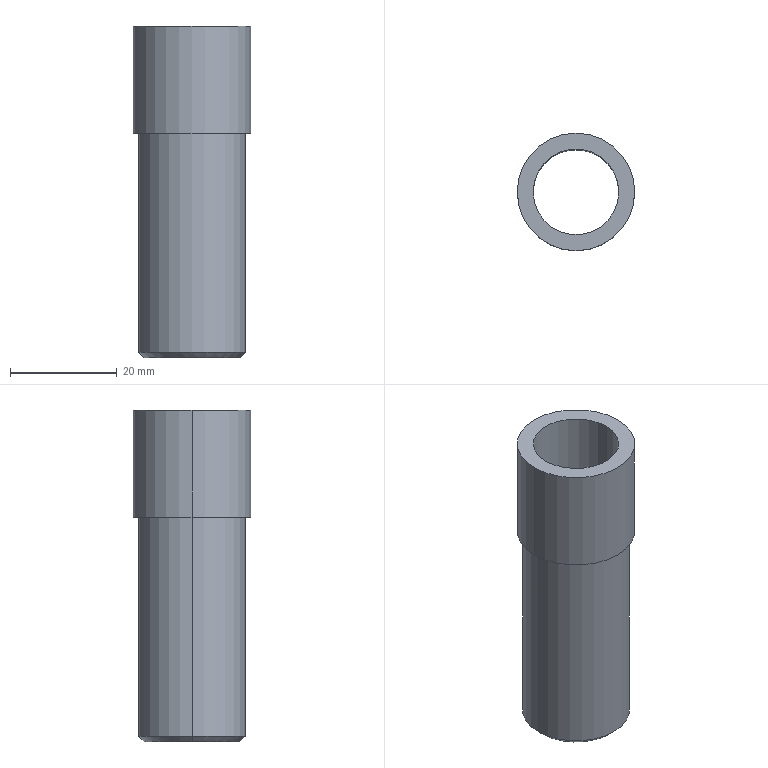Part | SolidWorks | features BaseBody 1 | 1 solid | 11 faces | box 22 x 22 x 62 mm | volume 8301 mm3 | cylinder 6 | plane 3 | cone 2 | commonest cylinder face diameters 16 x2 20 x2 22 x2
STEP:
#1=CARTESIAN_POINT('',(8.,0.,0.));
#2=VERTEX_POINT('',#1);
#3=CARTESIAN_POINT('',(-8.,0.,0.));
#4=VERTEX_POINT('',#3);
#5=CARTESIAN_POINT('',(0.,0.,0.));
#6=DIRECTION('',(0.,0.,-1.));
#7=DIRECTION('',(-1.,0.,0.));
#8=AXIS2_PLACEMENT_3D('',#5,#6,#7);
#9=CIRCLE('',#8,8.);
#10=EDGE_CURVE('',#2,#4,#9,.T.);
#11=ORIENTED_EDGE('',*,*,#10,.F.);
#12=CARTESIAN_POINT('',(8.,0.,-62.));
#13=VERTEX_POINT('',#12);
#14=CARTESIAN_POINT('',(8.,0.,-31.));
#15=DIRECTION('',(0.,0.,-1.));
#16=VECTOR('',#15,1000.);
#17=LINE('',#14,#16);
#18=EDGE_CURVE('',#2,#13,#17,.T.);
#19=ORIENTED_EDGE('',*,*,#18,.T.);
#20=CARTESIAN_POINT('',(-8.,0.,-62.));
#21=VERTEX_POINT('',#20);
#22=CARTESIAN_POINT('',(0.,0.,-62.));
#23=DIRECTION('',(0.,0.,1.));
#24=DIRECTION('',(-1.,0.,0.));
#25=AXIS2_PLACEMENT_3D('',#22,#23,#24);
#26=CIRCLE('',#25,8.);
#27=EDGE_CURVE('',#21,#13,#26,.T.);
#28=ORIENTED_EDGE('',*,*,#27,.F.);
#29=CARTESIAN_POINT('',(-8.,0.,-31.));
#30=DIRECTION('',(0.,0.,-1.));
#31=VECTOR('',#30,1000.);
#32=LINE('',#29,#31);
#33=EDGE_CURVE('',#4,#21,#32,.T.);
#34=ORIENTED_EDGE('',*,*,#33,.F.);
#35=EDGE_LOOP('',(#11,#19,#28,#34));
#36=FACE_OUTER_BOUND('',#35,.T.);
#37=CARTESIAN_POINT('',(0.,0.,-31.));
#38=DIRECTION('',(0.,0.,-1.));
#39=DIRECTION('',(-1.,0.,0.));
#40=AXIS2_PLACEMENT_3D('',#37,#38,#39);
#41=CYLINDRICAL_SURFACE('',#40,8.);
#42=ADVANCED_FACE('',(#36),#41,.F.);
#43=CARTESIAN_POINT('',(11.,0.,0.));
#44=VERTEX_POINT('',#43);
#45=CARTESIAN_POINT('',(-11.,0.,0.));
#46=VERTEX_POINT('',#45);
#47=CARTESIAN_POINT('',(0.,0.,0.));
#48=DIRECTION('',(0.,0.,1.));
#49=DIRECTION('',(-1.,0.,0.));
#50=AXIS2_PLACEMENT_3D('',#47,#48,#49);
#51=CIRCLE('',#50,11.);
#52=EDGE_CURVE('',#44,#46,#51,.T.);
#53=ORIENTED_EDGE('',*,*,#52,.F.);
#54=CARTESIAN_POINT('',(11.,0.,-20.));
#55=VERTEX_POINT('',#54);
#56=CARTESIAN_POINT('',(11.,0.,-10.));
#57=DIRECTION('',(0.,0.,-1.));
#58=VECTOR('',#57,1000.);
#59=LINE('',#56,#58);
#60=EDGE_CURVE('',#44,#55,#59,.T.);
#61=ORIENTED_EDGE('',*,*,#60,.T.);
#62=CARTESIAN_POINT('',(-11.,0.,-20.));
#63=VERTEX_POINT('',#62);
#64=CARTESIAN_POINT('',(0.,0.,-20.));
#65=DIRECTION('',(0.,0.,1.));
#66=DIRECTION('',(-1.,0.,0.));
#67=AXIS2_PLACEMENT_3D('',#64,#65,#66);
#68=CIRCLE('',#67,11.);
#69=EDGE_CURVE('',#55,#63,#68,.T.);
#70=ORIENTED_EDGE('',*,*,#69,.T.);
#71=CARTESIAN_POINT('',(-11.,0.,-10.));
#72=DIRECTION('',(0.,0.,-1.));
#73=VECTOR('',#72,1000.);
#74=LINE('',#71,#73);
#75=EDGE_CURVE('',#46,#63,#74,.T.);
#76=ORIENTED_EDGE('',*,*,#75,.F.);
#77=EDGE_LOOP('',(#53,#61,#70,#76));
#78=FACE_OUTER_BOUND('',#77,.T.);
#79=CARTESIAN_POINT('',(0.,0.,-10.));
#80=DIRECTION('',(0.,0.,-1.));
#81=DIRECTION('',(-1.,0.,0.));
#82=AXIS2_PLACEMENT_3D('',#79,#80,#81);
#83=CYLINDRICAL_SURFACE('',#82,11.);
#84=ADVANCED_FACE('',(#78),#83,.T.);
#85=CARTESIAN_POINT('',(-9.,0.,-62.));
#86=VERTEX_POINT('',#85);
#87=CARTESIAN_POINT('',(9.,0.,-62.));
#88=VERTEX_POINT('',#87);
#89=CARTESIAN_POINT('',(0.,0.,-62.));
#90=DIRECTION('',(0.,0.,-1.));
#91=DIRECTION('',(1.,0.,0.));
#92=AXIS2_PLACEMENT_3D('',#89,#90,#91);
#93=CIRCLE('',#92,9.);
#94=EDGE_CURVE('',#86,#88,#93,.T.);
#95=ORIENTED_EDGE('',*,*,#94,.F.);
#96=CARTESIAN_POINT('',(-10.,0.,-61.));
#97=VERTEX_POINT('',#96);
#98=CARTESIAN_POINT('',(-10.,0.,-61.));
#99=DIRECTION('',(-0.7071,0.,0.7071));
#100=VECTOR('',#99,1000.);
#101=LINE('',#98,#100);
#102=EDGE_CURVE('',#86,#97,#101,.T.);
#103=ORIENTED_EDGE('',*,*,#102,.T.);
#104=CARTESIAN_POINT('',(10.,0.,-61.));
#105=VERTEX_POINT('',#104);
#106=CARTESIAN_POINT('',(0.,0.,-61.));
#107=DIRECTION('',(0.,0.,-1.));
#108=DIRECTION('',(1.,0.,0.));
#109=AXIS2_PLACEMENT_3D('',#106,#107,#108);
#110=CIRCLE('',#109,10.);
#111=EDGE_CURVE('',#97,#105,#110,.T.);
#112=ORIENTED_EDGE('',*,*,#111,.T.);
#113=CARTESIAN_POINT('',(10.,0.,-61.));
#114=DIRECTION('',(0.7071,0.,0.7071));
#115=VECTOR('',#114,1000.);
#116=LINE('',#113,#115);
#117=EDGE_CURVE('',#88,#105,#116,.T.);
#118=ORIENTED_EDGE('',*,*,#117,.F.);
#119=EDGE_LOOP('',(#95,#103,#112,#118));
#120=FACE_OUTER_BOUND('',#119,.T.);
#121=CARTESIAN_POINT('',(0.,0.,-61.));
#122=DIRECTION('',(0.,0.,1.));
#123=DIRECTION('',(1.,0.,0.));
#124=AXIS2_PLACEMENT_3D('',#121,#122,#123);
#125=CONICAL_SURFACE('',#124,10.,0.7854);
#126=ADVANCED_FACE('',(#120),#125,.T.);
#127=CARTESIAN_POINT('',(10.,0.,-20.));
#128=VERTEX_POINT('',#127);
#129=CARTESIAN_POINT('',(-10.,0.,-20.));
#130=VERTEX_POINT('',#129);
#131=CARTESIAN_POINT('',(0.,0.,-20.));
#132=DIRECTION('',(0.,0.,1.));
#133=DIRECTION('',(-1.,0.,0.));
#134=AXIS2_PLACEMENT_3D('',#131,#132,#133);
#135=CIRCLE('',#134,10.);
#136=EDGE_CURVE('',#128,#130,#135,.T.);
#137=ORIENTED_EDGE('',*,*,#136,.F.);
#138=CARTESIAN_POINT('',(10.,0.,-41.));
#139=DIRECTION('',(0.,0.,-1.));
#140=VECTOR('',#139,1000.);
#141=LINE('',#138,#140);
#142=EDGE_CURVE('',#128,#105,#141,.T.);
#143=ORIENTED_EDGE('',*,*,#142,.T.);
#144=ORIENTED_EDGE('',*,*,#111,.F.);
#145=CARTESIAN_POINT('',(-10.,0.,-41.));
#146=DIRECTION('',(0.,0.,-1.));
#147=VECTOR('',#146,1000.);
#148=LINE('',#145,#147);
#149=EDGE_CURVE('',#130,#97,#148,.T.);
#150=ORIENTED_EDGE('',*,*,#149,.F.);
#151=EDGE_LOOP('',(#137,#143,#144,#150));
#152=FACE_OUTER_BOUND('',#151,.T.);
#153=CARTESIAN_POINT('',(0.,0.,-41.));
#154=DIRECTION('',(0.,0.,-1.));
#155=DIRECTION('',(-1.,0.,0.));
#156=AXIS2_PLACEMENT_3D('',#153,#154,#155);
#157=CYLINDRICAL_SURFACE('',#156,10.);
#158=ADVANCED_FACE('',(#152),#157,.T.);
#159=ORIENTED_EDGE('',*,*,#18,.F.);
#160=CARTESIAN_POINT('',(0.,0.,0.));
#161=DIRECTION('',(0.,0.,-1.));
#162=DIRECTION('',(-1.,0.,0.));
#163=AXIS2_PLACEMENT_3D('',#160,#161,#162);
#164=CIRCLE('',#163,8.);
#165=EDGE_CURVE('',#4,#2,#164,.T.);
#166=ORIENTED_EDGE('',*,*,#165,.F.);
#167=ORIENTED_EDGE('',*,*,#33,.T.);
#168=CARTESIAN_POINT('',(0.,0.,-62.));
#169=DIRECTION('',(0.,0.,1.));
#170=DIRECTION('',(-1.,0.,0.));
#171=AXIS2_PLACEMENT_3D('',#168,#169,#170);
#172=CIRCLE('',#171,8.);
#173=EDGE_CURVE('',#13,#21,#172,.T.);
#174=ORIENTED_EDGE('',*,*,#173,.F.);
#175=EDGE_LOOP('',(#159,#166,#167,#174));
#176=FACE_OUTER_BOUND('',#175,.T.);
#177=CARTESIAN_POINT('',(0.,0.,-31.));
#178=DIRECTION('',(0.,0.,-1.));
#179=DIRECTION('',(-1.,0.,0.));
#180=AXIS2_PLACEMENT_3D('',#177,#178,#179);
#181=CYLINDRICAL_SURFACE('',#180,8.);
#182=ADVANCED_FACE('',(#176),#181,.F.);
#183=ORIENTED_EDGE('',*,*,#165,.T.);
#184=ORIENTED_EDGE('',*,*,#10,.T.);
#185=EDGE_LOOP('',(#183,#184));
#186=FACE_BOUND('',#185,.T.);
#187=CARTESIAN_POINT('',(0.,0.,0.));
#188=DIRECTION('',(0.,0.,1.));
#189=DIRECTION('',(-1.,0.,0.));
#190=AXIS2_PLACEMENT_3D('',#187,#188,#189);
#191=CIRCLE('',#190,11.);
#192=EDGE_CURVE('',#46,#44,#191,.T.);
#193=ORIENTED_EDGE('',*,*,#192,.T.);
#194=ORIENTED_EDGE('',*,*,#52,.T.);
#195=EDGE_LOOP('',(#193,#194));
#196=FACE_OUTER_BOUND('',#195,.T.);
#197=CARTESIAN_POINT('',(-11.,0.,0.));
#198=DIRECTION('',(0.,0.,1.));
#199=DIRECTION('',(1.,0.,0.));
#200=AXIS2_PLACEMENT_3D('',#197,#198,#199);
#201=PLANE('',#200);
#202=ADVANCED_FACE('',(#186,#196),#201,.T.);
#203=ORIENTED_EDGE('',*,*,#27,.T.);
#204=ORIENTED_EDGE('',*,*,#173,.T.);
#205=EDGE_LOOP('',(#203,#204));
#206=FACE_BOUND('',#205,.T.);
#207=CARTESIAN_POINT('',(0.,0.,-62.));
#208=DIRECTION('',(0.,0.,-1.));
#209=DIRECTION('',(1.,0.,0.));
#210=AXIS2_PLACEMENT_3D('',#207,#208,#209);
#211=CIRCLE('',#210,9.);
#212=EDGE_CURVE('',#88,#86,#211,.T.);
#213=ORIENTED_EDGE('',*,*,#212,.T.);
#214=ORIENTED_EDGE('',*,*,#94,.T.);
#215=EDGE_LOOP('',(#213,#214));
#216=FACE_OUTER_BOUND('',#215,.T.);
#217=CARTESIAN_POINT('',(-8.,0.,-62.));
#218=DIRECTION('',(0.,0.,-1.));
#219=DIRECTION('',(-1.,0.,0.));
#220=AXIS2_PLACEMENT_3D('',#217,#218,#219);
#221=PLANE('',#220);
#222=ADVANCED_FACE('',(#206,#216),#221,.T.);
#223=ORIENTED_EDGE('',*,*,#60,.F.);
#224=ORIENTED_EDGE('',*,*,#192,.F.);
#225=ORIENTED_EDGE('',*,*,#75,.T.);
#226=CARTESIAN_POINT('',(0.,0.,-20.));
#227=DIRECTION('',(0.,0.,1.));
#228=DIRECTION('',(-1.,0.,0.));
#229=AXIS2_PLACEMENT_3D('',#226,#227,#228);
#230=CIRCLE('',#229,11.);
#231=EDGE_CURVE('',#63,#55,#230,.T.);
#232=ORIENTED_EDGE('',*,*,#231,.T.);
#233=EDGE_LOOP('',(#223,#224,#225,#232));
#234=FACE_OUTER_BOUND('',#233,.T.);
#235=CARTESIAN_POINT('',(0.,0.,-10.));
#236=DIRECTION('',(0.,0.,-1.));
#237=DIRECTION('',(-1.,0.,0.));
#238=AXIS2_PLACEMENT_3D('',#235,#236,#237);
#239=CYLINDRICAL_SURFACE('',#238,11.);
#240=ADVANCED_FACE('',(#234),#239,.T.);
#241=ORIENTED_EDGE('',*,*,#102,.F.);
#242=ORIENTED_EDGE('',*,*,#212,.F.);
#243=ORIENTED_EDGE('',*,*,#117,.T.);
#244=CARTESIAN_POINT('',(0.,0.,-61.));
#245=DIRECTION('',(0.,0.,-1.));
#246=DIRECTION('',(1.,0.,0.));
#247=AXIS2_PLACEMENT_3D('',#244,#245,#246);
#248=CIRCLE('',#247,10.);
#249=EDGE_CURVE('',#105,#97,#248,.T.);
#250=ORIENTED_EDGE('',*,*,#249,.T.);
#251=EDGE_LOOP('',(#241,#242,#243,#250));
#252=FACE_OUTER_BOUND('',#251,.T.);
#253=CARTESIAN_POINT('',(0.,0.,-61.));
#254=DIRECTION('',(0.,0.,1.));
#255=DIRECTION('',(1.,0.,0.));
#256=AXIS2_PLACEMENT_3D('',#253,#254,#255);
#257=CONICAL_SURFACE('',#256,10.,0.7854);
#258=ADVANCED_FACE('',(#252),#257,.T.);
#259=CARTESIAN_POINT('',(0.,0.,-20.));
#260=DIRECTION('',(0.,0.,1.));
#261=DIRECTION('',(-1.,0.,0.));
#262=AXIS2_PLACEMENT_3D('',#259,#260,#261);
#263=CIRCLE('',#262,10.);
#264=EDGE_CURVE('',#130,#128,#263,.T.);
#265=ORIENTED_EDGE('',*,*,#264,.T.);
#266=ORIENTED_EDGE('',*,*,#136,.T.);
#267=EDGE_LOOP('',(#265,#266));
#268=FACE_BOUND('',#267,.T.);
#269=ORIENTED_EDGE('',*,*,#231,.F.);
#270=ORIENTED_EDGE('',*,*,#69,.F.);
#271=EDGE_LOOP('',(#269,#270));
#272=FACE_OUTER_BOUND('',#271,.T.);
#273=CARTESIAN_POINT('',(-10.,0.,-20.));
#274=DIRECTION('',(0.,0.,-1.));
#275=DIRECTION('',(-1.,0.,0.));
#276=AXIS2_PLACEMENT_3D('',#273,#274,#275);
#277=PLANE('',#276);
#278=ADVANCED_FACE('',(#268,#272),#277,.T.);
#279=ORIENTED_EDGE('',*,*,#142,.F.);
#280=ORIENTED_EDGE('',*,*,#264,.F.);
#281=ORIENTED_EDGE('',*,*,#149,.T.);
#282=ORIENTED_EDGE('',*,*,#249,.F.);
#283=EDGE_LOOP('',(#279,#280,#281,#282));
#284=FACE_OUTER_BOUND('',#283,.T.);
#285=CARTESIAN_POINT('',(0.,0.,-41.));
#286=DIRECTION('',(0.,0.,-1.));
#287=DIRECTION('',(-1.,0.,0.));
#288=AXIS2_PLACEMENT_3D('',#285,#286,#287);
#289=CYLINDRICAL_SURFACE('',#288,10.);
#290=ADVANCED_FACE('',(#284),#289,.T.);
#291=CLOSED_SHELL('',(#42,#84,#126,#158,#182,#202,#222,#240,#258,#278,#290));
#292=MANIFOLD_SOLID_BREP('',#291);
#293=CARTESIAN_POINT('',(0.,0.,0.));
#294=DIRECTION('',(0.,0.,1.));
#295=DIRECTION('',(1.,0.,0.));
#296=AXIS2_PLACEMENT_3D('',#293,#294,#295);
#297=(LENGTH_UNIT()NAMED_UNIT(*)SI_UNIT(.MILLI.,.METRE.));
#298=UNCERTAINTY_MEASURE_WITH_UNIT(LENGTH_MEASURE(0.00001),#297,'','');
#299=(NAMED_UNIT(*)PLANE_ANGLE_UNIT()SI_UNIT($,.RADIAN.));
#300=(NAMED_UNIT(*)SI_UNIT($,.STERADIAN.)SOLID_ANGLE_UNIT());
#301=(GEOMETRIC_REPRESENTATION_CONTEXT(3)GLOBAL_UNCERTAINTY_ASSIGNED_CONTEXT((#298))GLOBAL_UNIT_ASSIGNED_CONTEXT((#297,#299,#300))REPRESENTATION_CONTEXT('',''));
#302=ADVANCED_BREP_SHAPE_REPRESENTATION('',(#292,#296),#301);